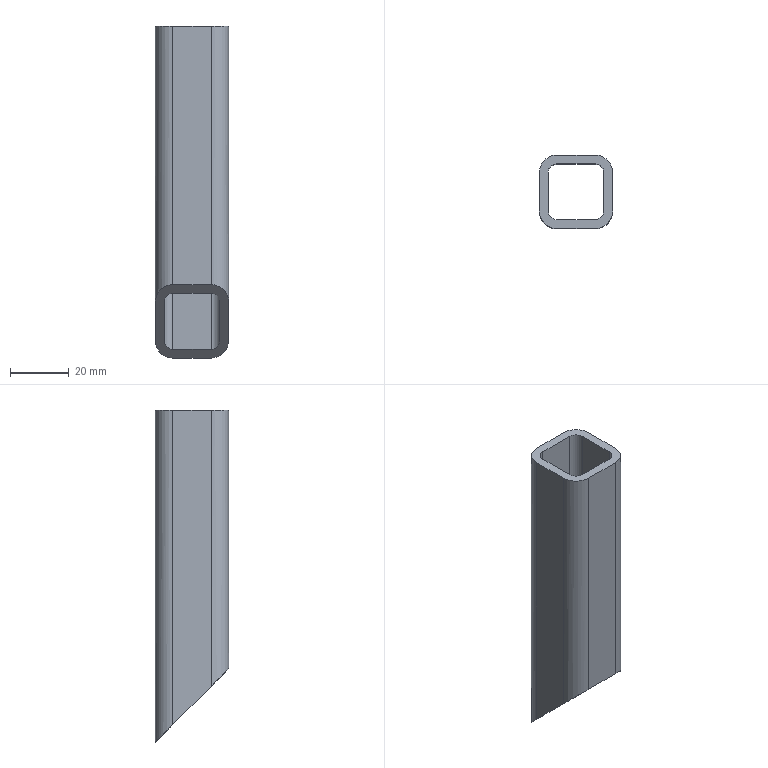Part | STEP file | ISO 10799-2 25x25x3 1784907954311 | 1 solid | 18 faces | box 25 x 25 x 113.072 mm | volume 24220 mm3 | plane 10 | cylinder 8 | commonest cylinder face diameters 6 x4 12 x4
STEP:
#1=CARTESIAN_POINT('',(12.5,-6.5,6.5));
#2=VERTEX_POINT('',#1);
#3=CARTESIAN_POINT('',(12.5,6.5,-6.5));
#4=VERTEX_POINT('',#3);
#5=CARTESIAN_POINT('',(12.5,1.625,-1.625));
#6=DIRECTION('',(0.,0.7071,-0.7071));
#7=VECTOR('',#6,10.);
#8=LINE('',#5,#7);
#9=EDGE_CURVE('',#2,#4,#8,.T.);
#10=ORIENTED_EDGE('',*,*,#9,.F.);
#11=CARTESIAN_POINT('',(6.5,-12.5,12.5));
#12=VERTEX_POINT('',#11);
#13=CARTESIAN_POINT('',(6.5,-6.5,6.5));
#14=DIRECTION('',(0.,0.7071,0.7071));
#15=DIRECTION('',(0.,0.7071,-0.7071));
#16=AXIS2_PLACEMENT_3D('',#13,#14,#15);
#17=ELLIPSE('',#16,8.485,6.);
#18=EDGE_CURVE('',#12,#2,#17,.T.);
#19=ORIENTED_EDGE('',*,*,#18,.F.);
#20=CARTESIAN_POINT('',(-6.5,-12.5,12.5));
#21=VERTEX_POINT('',#20);
#22=CARTESIAN_POINT('',(3.25,-12.5,12.5));
#23=DIRECTION('',(1.,0.,0.));
#24=VECTOR('',#23,10.);
#25=LINE('',#22,#24);
#26=EDGE_CURVE('',#21,#12,#25,.T.);
#27=ORIENTED_EDGE('',*,*,#26,.F.);
#28=CARTESIAN_POINT('',(-12.5,-6.5,6.5));
#29=VERTEX_POINT('',#28);
#30=CARTESIAN_POINT('',(-6.5,-6.5,6.5));
#31=DIRECTION('',(0.,0.7071,0.7071));
#32=DIRECTION('',(0.,0.7071,-0.7071));
#33=AXIS2_PLACEMENT_3D('',#30,#31,#32);
#34=ELLIPSE('',#33,8.485,6.);
#35=EDGE_CURVE('',#29,#21,#34,.T.);
#36=ORIENTED_EDGE('',*,*,#35,.F.);
#37=CARTESIAN_POINT('',(-12.5,6.5,-6.5));
#38=VERTEX_POINT('',#37);
#39=CARTESIAN_POINT('',(-12.5,-1.625,1.625));
#40=DIRECTION('',(0.,-0.7071,0.7071));
#41=VECTOR('',#40,10.);
#42=LINE('',#39,#41);
#43=EDGE_CURVE('',#38,#29,#42,.T.);
#44=ORIENTED_EDGE('',*,*,#43,.F.);
#45=CARTESIAN_POINT('',(-6.5,12.5,-12.5));
#46=VERTEX_POINT('',#45);
#47=CARTESIAN_POINT('',(-6.5,6.5,-6.5));
#48=DIRECTION('',(0.,0.7071,0.7071));
#49=DIRECTION('',(0.,-0.7071,0.7071));
#50=AXIS2_PLACEMENT_3D('',#47,#48,#49);
#51=ELLIPSE('',#50,8.485,6.);
#52=EDGE_CURVE('',#46,#38,#51,.T.);
#53=ORIENTED_EDGE('',*,*,#52,.F.);
#54=CARTESIAN_POINT('',(6.5,12.5,-12.5));
#55=VERTEX_POINT('',#54);
#56=CARTESIAN_POINT('',(-3.25,12.5,-12.5));
#57=DIRECTION('',(1.,0.,0.));
#58=VECTOR('',#57,10.);
#59=LINE('',#56,#58);
#60=EDGE_CURVE('',#46,#55,#59,.T.);
#61=ORIENTED_EDGE('',*,*,#60,.T.);
#62=CARTESIAN_POINT('',(6.5,6.5,-6.5));
#63=DIRECTION('',(0.,0.7071,0.7071));
#64=DIRECTION('',(0.,-0.7071,0.7071));
#65=AXIS2_PLACEMENT_3D('',#62,#63,#64);
#66=ELLIPSE('',#65,8.485,6.);
#67=EDGE_CURVE('',#4,#55,#66,.T.);
#68=ORIENTED_EDGE('',*,*,#67,.F.);
#69=EDGE_LOOP('',(#10,#19,#27,#36,#44,#53,#61,#68));
#70=FACE_OUTER_BOUND('',#69,.T.);
#71=CARTESIAN_POINT('',(6.5,-9.5,9.5));
#72=VERTEX_POINT('',#71);
#73=CARTESIAN_POINT('',(-6.5,-9.5,9.5));
#74=VERTEX_POINT('',#73);
#75=CARTESIAN_POINT('',(3.25,-9.5,9.5));
#76=DIRECTION('',(-1.,0.,0.));
#77=VECTOR('',#76,10.);
#78=LINE('',#75,#77);
#79=EDGE_CURVE('',#72,#74,#78,.T.);
#80=ORIENTED_EDGE('',*,*,#79,.F.);
#81=CARTESIAN_POINT('',(9.5,-6.5,6.5));
#82=VERTEX_POINT('',#81);
#83=CARTESIAN_POINT('',(6.5,-6.5,6.5));
#84=DIRECTION('',(0.,-0.7071,-0.7071));
#85=DIRECTION('',(0.,0.7071,-0.7071));
#86=AXIS2_PLACEMENT_3D('',#83,#84,#85);
#87=ELLIPSE('',#86,4.243,3.);
#88=EDGE_CURVE('',#82,#72,#87,.T.);
#89=ORIENTED_EDGE('',*,*,#88,.F.);
#90=CARTESIAN_POINT('',(9.5,6.5,-6.5));
#91=VERTEX_POINT('',#90);
#92=CARTESIAN_POINT('',(9.5,1.625,-1.625));
#93=DIRECTION('',(0.,-0.7071,0.7071));
#94=VECTOR('',#93,10.);
#95=LINE('',#92,#94);
#96=EDGE_CURVE('',#91,#82,#95,.T.);
#97=ORIENTED_EDGE('',*,*,#96,.F.);
#98=CARTESIAN_POINT('',(6.5,9.5,-9.5));
#99=VERTEX_POINT('',#98);
#100=CARTESIAN_POINT('',(6.5,6.5,-6.5));
#101=DIRECTION('',(0.,-0.7071,-0.7071));
#102=DIRECTION('',(0.,-0.7071,0.7071));
#103=AXIS2_PLACEMENT_3D('',#100,#101,#102);
#104=ELLIPSE('',#103,4.243,3.);
#105=EDGE_CURVE('',#99,#91,#104,.T.);
#106=ORIENTED_EDGE('',*,*,#105,.F.);
#107=CARTESIAN_POINT('',(-6.5,9.5,-9.5));
#108=VERTEX_POINT('',#107);
#109=CARTESIAN_POINT('',(-3.25,9.5,-9.5));
#110=DIRECTION('',(1.,0.,0.));
#111=VECTOR('',#110,10.);
#112=LINE('',#109,#111);
#113=EDGE_CURVE('',#108,#99,#112,.T.);
#114=ORIENTED_EDGE('',*,*,#113,.F.);
#115=CARTESIAN_POINT('',(-9.5,6.5,-6.5));
#116=VERTEX_POINT('',#115);
#117=CARTESIAN_POINT('',(-6.5,6.5,-6.5));
#118=DIRECTION('',(0.,-0.7071,-0.7071));
#119=DIRECTION('',(0.,-0.7071,0.7071));
#120=AXIS2_PLACEMENT_3D('',#117,#118,#119);
#121=ELLIPSE('',#120,4.243,3.);
#122=EDGE_CURVE('',#116,#108,#121,.T.);
#123=ORIENTED_EDGE('',*,*,#122,.F.);
#124=CARTESIAN_POINT('',(-9.5,-6.5,6.5));
#125=VERTEX_POINT('',#124);
#126=CARTESIAN_POINT('',(-9.5,-1.625,1.625));
#127=DIRECTION('',(0.,0.7071,-0.7071));
#128=VECTOR('',#127,10.);
#129=LINE('',#126,#128);
#130=EDGE_CURVE('',#125,#116,#129,.T.);
#131=ORIENTED_EDGE('',*,*,#130,.F.);
#132=CARTESIAN_POINT('',(-6.5,-6.5,6.5));
#133=DIRECTION('',(0.,-0.7071,-0.7071));
#134=DIRECTION('',(0.,0.7071,-0.7071));
#135=AXIS2_PLACEMENT_3D('',#132,#133,#134);
#136=ELLIPSE('',#135,4.243,3.);
#137=EDGE_CURVE('',#74,#125,#136,.T.);
#138=ORIENTED_EDGE('',*,*,#137,.F.);
#139=EDGE_LOOP('',(#80,#89,#97,#106,#114,#123,#131,#138));
#140=FACE_BOUND('',#139,.T.);
#141=CARTESIAN_POINT('',(0.,0.,0.));
#142=DIRECTION('',(0.,0.7071,0.7071));
#143=DIRECTION('',(1.,0.,0.));
#144=AXIS2_PLACEMENT_3D('',#141,#142,#143);
#145=PLANE('',#144);
#146=ADVANCED_FACE('',(#70,#140),#145,.F.);
#147=ORIENTED_EDGE('',*,*,#113,.T.);
#148=CARTESIAN_POINT('',(6.5,9.5,100.572));
#149=VERTEX_POINT('',#148);
#150=CARTESIAN_POINT('',(6.5,9.5,0.));
#151=DIRECTION('',(0.,0.,-1.));
#152=VECTOR('',#151,10.);
#153=LINE('',#150,#152);
#154=EDGE_CURVE('',#149,#99,#153,.T.);
#155=ORIENTED_EDGE('',*,*,#154,.F.);
#156=CARTESIAN_POINT('',(-6.5,9.5,100.572));
#157=VERTEX_POINT('',#156);
#158=CARTESIAN_POINT('',(-3.25,9.5,100.572));
#159=DIRECTION('',(-1.,0.,0.));
#160=VECTOR('',#159,10.);
#161=LINE('',#158,#160);
#162=EDGE_CURVE('',#149,#157,#161,.T.);
#163=ORIENTED_EDGE('',*,*,#162,.T.);
#164=CARTESIAN_POINT('',(-6.5,9.5,0.));
#165=DIRECTION('',(0.,0.,-1.));
#166=VECTOR('',#165,10.);
#167=LINE('',#164,#166);
#168=EDGE_CURVE('',#157,#108,#167,.T.);
#169=ORIENTED_EDGE('',*,*,#168,.T.);
#170=EDGE_LOOP('',(#147,#155,#163,#169));
#171=FACE_OUTER_BOUND('',#170,.T.);
#172=CARTESIAN_POINT('',(-6.5,9.5,0.));
#173=DIRECTION('',(0.,1.,0.));
#174=DIRECTION('',(0.,0.,1.));
#175=AXIS2_PLACEMENT_3D('',#172,#173,#174);
#176=PLANE('',#175);
#177=ADVANCED_FACE('',(#171),#176,.F.);
#178=ORIENTED_EDGE('',*,*,#105,.T.);
#179=CARTESIAN_POINT('',(9.5,6.5,100.572));
#180=VERTEX_POINT('',#179);
#181=CARTESIAN_POINT('',(9.5,6.5,0.));
#182=DIRECTION('',(0.,0.,-1.));
#183=VECTOR('',#182,10.);
#184=LINE('',#181,#183);
#185=EDGE_CURVE('',#180,#91,#184,.T.);
#186=ORIENTED_EDGE('',*,*,#185,.F.);
#187=CARTESIAN_POINT('',(6.5,6.5,100.572));
#188=DIRECTION('',(0.,0.,1.));
#189=DIRECTION('',(-1.,0.,0.));
#190=AXIS2_PLACEMENT_3D('',#187,#188,#189);
#191=CIRCLE('',#190,3.);
#192=EDGE_CURVE('',#180,#149,#191,.T.);
#193=ORIENTED_EDGE('',*,*,#192,.T.);
#194=ORIENTED_EDGE('',*,*,#154,.T.);
#195=EDGE_LOOP('',(#178,#186,#193,#194));
#196=FACE_OUTER_BOUND('',#195,.T.);
#197=CARTESIAN_POINT('',(6.5,6.5,0.));
#198=DIRECTION('',(0.,0.,1.));
#199=DIRECTION('',(-1.,0.,0.));
#200=AXIS2_PLACEMENT_3D('',#197,#198,#199);
#201=CYLINDRICAL_SURFACE('',#200,3.);
#202=ADVANCED_FACE('',(#196),#201,.F.);
#203=ORIENTED_EDGE('',*,*,#96,.T.);
#204=CARTESIAN_POINT('',(9.5,-6.5,100.572));
#205=VERTEX_POINT('',#204);
#206=CARTESIAN_POINT('',(9.5,-6.5,0.));
#207=DIRECTION('',(0.,0.,-1.));
#208=VECTOR('',#207,10.);
#209=LINE('',#206,#208);
#210=EDGE_CURVE('',#205,#82,#209,.T.);
#211=ORIENTED_EDGE('',*,*,#210,.F.);
#212=CARTESIAN_POINT('',(9.5,3.25,100.572));
#213=DIRECTION('',(0.,1.,0.));
#214=VECTOR('',#213,10.);
#215=LINE('',#212,#214);
#216=EDGE_CURVE('',#205,#180,#215,.T.);
#217=ORIENTED_EDGE('',*,*,#216,.T.);
#218=ORIENTED_EDGE('',*,*,#185,.T.);
#219=EDGE_LOOP('',(#203,#211,#217,#218));
#220=FACE_OUTER_BOUND('',#219,.T.);
#221=CARTESIAN_POINT('',(9.5,6.5,0.));
#222=DIRECTION('',(1.,0.,0.));
#223=DIRECTION('',(0.,0.,-1.));
#224=AXIS2_PLACEMENT_3D('',#221,#222,#223);
#225=PLANE('',#224);
#226=ADVANCED_FACE('',(#220),#225,.F.);
#227=ORIENTED_EDGE('',*,*,#88,.T.);
#228=CARTESIAN_POINT('',(6.5,-9.5,100.572));
#229=VERTEX_POINT('',#228);
#230=CARTESIAN_POINT('',(6.5,-9.5,0.));
#231=DIRECTION('',(0.,0.,-1.));
#232=VECTOR('',#231,10.);
#233=LINE('',#230,#232);
#234=EDGE_CURVE('',#229,#72,#233,.T.);
#235=ORIENTED_EDGE('',*,*,#234,.F.);
#236=CARTESIAN_POINT('',(6.5,-6.5,100.572));
#237=DIRECTION('',(0.,0.,1.));
#238=DIRECTION('',(0.,1.,0.));
#239=AXIS2_PLACEMENT_3D('',#236,#237,#238);
#240=CIRCLE('',#239,3.);
#241=EDGE_CURVE('',#229,#205,#240,.T.);
#242=ORIENTED_EDGE('',*,*,#241,.T.);
#243=ORIENTED_EDGE('',*,*,#210,.T.);
#244=EDGE_LOOP('',(#227,#235,#242,#243));
#245=FACE_OUTER_BOUND('',#244,.T.);
#246=CARTESIAN_POINT('',(6.5,-6.5,0.));
#247=DIRECTION('',(0.,0.,1.));
#248=DIRECTION('',(0.,1.,0.));
#249=AXIS2_PLACEMENT_3D('',#246,#247,#248);
#250=CYLINDRICAL_SURFACE('',#249,3.);
#251=ADVANCED_FACE('',(#245),#250,.F.);
#252=ORIENTED_EDGE('',*,*,#43,.T.);
#253=CARTESIAN_POINT('',(-12.5,-6.5,100.572));
#254=VERTEX_POINT('',#253);
#255=CARTESIAN_POINT('',(-12.5,-6.5,0.));
#256=DIRECTION('',(0.,0.,-1.));
#257=VECTOR('',#256,10.);
#258=LINE('',#255,#257);
#259=EDGE_CURVE('',#254,#29,#258,.T.);
#260=ORIENTED_EDGE('',*,*,#259,.F.);
#261=CARTESIAN_POINT('',(-12.5,6.5,100.572));
#262=VERTEX_POINT('',#261);
#263=CARTESIAN_POINT('',(-12.5,-3.25,100.572));
#264=DIRECTION('',(0.,1.,0.));
#265=VECTOR('',#264,10.);
#266=LINE('',#263,#265);
#267=EDGE_CURVE('',#254,#262,#266,.T.);
#268=ORIENTED_EDGE('',*,*,#267,.T.);
#269=CARTESIAN_POINT('',(-12.5,6.5,0.));
#270=DIRECTION('',(0.,0.,-1.));
#271=VECTOR('',#270,10.);
#272=LINE('',#269,#271);
#273=EDGE_CURVE('',#262,#38,#272,.T.);
#274=ORIENTED_EDGE('',*,*,#273,.T.);
#275=EDGE_LOOP('',(#252,#260,#268,#274));
#276=FACE_OUTER_BOUND('',#275,.T.);
#277=CARTESIAN_POINT('',(-12.5,-6.5,0.));
#278=DIRECTION('',(-1.,0.,0.));
#279=DIRECTION('',(0.,0.,1.));
#280=AXIS2_PLACEMENT_3D('',#277,#278,#279);
#281=PLANE('',#280);
#282=ADVANCED_FACE('',(#276),#281,.T.);
#283=ORIENTED_EDGE('',*,*,#35,.T.);
#284=CARTESIAN_POINT('',(-6.5,-12.5,100.572));
#285=VERTEX_POINT('',#284);
#286=CARTESIAN_POINT('',(-6.5,-12.5,0.));
#287=DIRECTION('',(0.,0.,1.));
#288=VECTOR('',#287,10.);
#289=LINE('',#286,#288);
#290=EDGE_CURVE('',#21,#285,#289,.T.);
#291=ORIENTED_EDGE('',*,*,#290,.T.);
#292=CARTESIAN_POINT('',(-6.5,-6.5,100.572));
#293=DIRECTION('',(0.,0.,-1.));
#294=DIRECTION('',(1.,0.,0.));
#295=AXIS2_PLACEMENT_3D('',#292,#293,#294);
#296=CIRCLE('',#295,6.);
#297=EDGE_CURVE('',#285,#254,#296,.T.);
#298=ORIENTED_EDGE('',*,*,#297,.T.);
#299=ORIENTED_EDGE('',*,*,#259,.T.);
#300=EDGE_LOOP('',(#283,#291,#298,#299));
#301=FACE_OUTER_BOUND('',#300,.T.);
#302=CARTESIAN_POINT('',(-6.5,-6.5,0.));
#303=DIRECTION('',(0.,0.,1.));
#304=DIRECTION('',(1.,0.,0.));
#305=AXIS2_PLACEMENT_3D('',#302,#303,#304);
#306=CYLINDRICAL_SURFACE('',#305,6.);
#307=ADVANCED_FACE('',(#301),#306,.T.);
#308=ORIENTED_EDGE('',*,*,#26,.T.);
#309=CARTESIAN_POINT('',(6.5,-12.5,100.572));
#310=VERTEX_POINT('',#309);
#311=CARTESIAN_POINT('',(6.5,-12.5,0.));
#312=DIRECTION('',(0.,0.,-1.));
#313=VECTOR('',#312,10.);
#314=LINE('',#311,#313);
#315=EDGE_CURVE('',#310,#12,#314,.T.);
#316=ORIENTED_EDGE('',*,*,#315,.F.);
#317=CARTESIAN_POINT('',(3.25,-12.5,100.572));
#318=DIRECTION('',(-1.,0.,0.));
#319=VECTOR('',#318,10.);
#320=LINE('',#317,#319);
#321=EDGE_CURVE('',#310,#285,#320,.T.);
#322=ORIENTED_EDGE('',*,*,#321,.T.);
#323=ORIENTED_EDGE('',*,*,#290,.F.);
#324=EDGE_LOOP('',(#308,#316,#322,#323));
#325=FACE_OUTER_BOUND('',#324,.T.);
#326=CARTESIAN_POINT('',(6.5,-12.5,0.));
#327=DIRECTION('',(0.,-1.,0.));
#328=DIRECTION('',(0.,0.,-1.));
#329=AXIS2_PLACEMENT_3D('',#326,#327,#328);
#330=PLANE('',#329);
#331=ADVANCED_FACE('',(#325),#330,.T.);
#332=ORIENTED_EDGE('',*,*,#18,.T.);
#333=CARTESIAN_POINT('',(12.5,-6.5,100.572));
#334=VERTEX_POINT('',#333);
#335=CARTESIAN_POINT('',(12.5,-6.5,0.));
#336=DIRECTION('',(0.,0.,-1.));
#337=VECTOR('',#336,10.);
#338=LINE('',#335,#337);
#339=EDGE_CURVE('',#334,#2,#338,.T.);
#340=ORIENTED_EDGE('',*,*,#339,.F.);
#341=CARTESIAN_POINT('',(6.5,-6.5,100.572));
#342=DIRECTION('',(0.,0.,-1.));
#343=DIRECTION('',(0.,1.,0.));
#344=AXIS2_PLACEMENT_3D('',#341,#342,#343);
#345=CIRCLE('',#344,6.);
#346=EDGE_CURVE('',#334,#310,#345,.T.);
#347=ORIENTED_EDGE('',*,*,#346,.T.);
#348=ORIENTED_EDGE('',*,*,#315,.T.);
#349=EDGE_LOOP('',(#332,#340,#347,#348));
#350=FACE_OUTER_BOUND('',#349,.T.);
#351=CARTESIAN_POINT('',(6.5,-6.5,0.));
#352=DIRECTION('',(0.,0.,1.));
#353=DIRECTION('',(0.,1.,0.));
#354=AXIS2_PLACEMENT_3D('',#351,#352,#353);
#355=CYLINDRICAL_SURFACE('',#354,6.);
#356=ADVANCED_FACE('',(#350),#355,.T.);
#357=ORIENTED_EDGE('',*,*,#79,.T.);
#358=CARTESIAN_POINT('',(-6.5,-9.5,100.572));
#359=VERTEX_POINT('',#358);
#360=CARTESIAN_POINT('',(-6.5,-9.5,0.));
#361=DIRECTION('',(0.,0.,-1.));
#362=VECTOR('',#361,10.);
#363=LINE('',#360,#362);
#364=EDGE_CURVE('',#359,#74,#363,.T.);
#365=ORIENTED_EDGE('',*,*,#364,.F.);
#366=CARTESIAN_POINT('',(3.25,-9.5,100.572));
#367=DIRECTION('',(1.,0.,0.));
#368=VECTOR('',#367,10.);
#369=LINE('',#366,#368);
#370=EDGE_CURVE('',#359,#229,#369,.T.);
#371=ORIENTED_EDGE('',*,*,#370,.T.);
#372=ORIENTED_EDGE('',*,*,#234,.T.);
#373=EDGE_LOOP('',(#357,#365,#371,#372));
#374=FACE_OUTER_BOUND('',#373,.T.);
#375=CARTESIAN_POINT('',(6.5,-9.5,0.));
#376=DIRECTION('',(0.,-1.,0.));
#377=DIRECTION('',(0.,0.,-1.));
#378=AXIS2_PLACEMENT_3D('',#375,#376,#377);
#379=PLANE('',#378);
#380=ADVANCED_FACE('',(#374),#379,.F.);
#381=ORIENTED_EDGE('',*,*,#9,.T.);
#382=CARTESIAN_POINT('',(12.5,6.5,100.572));
#383=VERTEX_POINT('',#382);
#384=CARTESIAN_POINT('',(12.5,6.5,0.));
#385=DIRECTION('',(0.,0.,-1.));
#386=VECTOR('',#385,10.);
#387=LINE('',#384,#386);
#388=EDGE_CURVE('',#383,#4,#387,.T.);
#389=ORIENTED_EDGE('',*,*,#388,.F.);
#390=CARTESIAN_POINT('',(12.5,3.25,100.572));
#391=DIRECTION('',(0.,-1.,0.));
#392=VECTOR('',#391,10.);
#393=LINE('',#390,#392);
#394=EDGE_CURVE('',#383,#334,#393,.T.);
#395=ORIENTED_EDGE('',*,*,#394,.T.);
#396=ORIENTED_EDGE('',*,*,#339,.T.);
#397=EDGE_LOOP('',(#381,#389,#395,#396));
#398=FACE_OUTER_BOUND('',#397,.T.);
#399=CARTESIAN_POINT('',(12.5,6.5,0.));
#400=DIRECTION('',(1.,0.,0.));
#401=DIRECTION('',(0.,0.,-1.));
#402=AXIS2_PLACEMENT_3D('',#399,#400,#401);
#403=PLANE('',#402);
#404=ADVANCED_FACE('',(#398),#403,.T.);
#405=ORIENTED_EDGE('',*,*,#137,.T.);
#406=CARTESIAN_POINT('',(-9.5,-6.5,100.572));
#407=VERTEX_POINT('',#406);
#408=CARTESIAN_POINT('',(-9.5,-6.5,0.));
#409=DIRECTION('',(0.,0.,-1.));
#410=VECTOR('',#409,10.);
#411=LINE('',#408,#410);
#412=EDGE_CURVE('',#407,#125,#411,.T.);
#413=ORIENTED_EDGE('',*,*,#412,.F.);
#414=CARTESIAN_POINT('',(-6.5,-6.5,100.572));
#415=DIRECTION('',(0.,0.,1.));
#416=DIRECTION('',(1.,0.,0.));
#417=AXIS2_PLACEMENT_3D('',#414,#415,#416);
#418=CIRCLE('',#417,3.);
#419=EDGE_CURVE('',#407,#359,#418,.T.);
#420=ORIENTED_EDGE('',*,*,#419,.T.);
#421=ORIENTED_EDGE('',*,*,#364,.T.);
#422=EDGE_LOOP('',(#405,#413,#420,#421));
#423=FACE_OUTER_BOUND('',#422,.T.);
#424=CARTESIAN_POINT('',(-6.5,-6.5,0.));
#425=DIRECTION('',(0.,0.,1.));
#426=DIRECTION('',(1.,0.,0.));
#427=AXIS2_PLACEMENT_3D('',#424,#425,#426);
#428=CYLINDRICAL_SURFACE('',#427,3.);
#429=ADVANCED_FACE('',(#423),#428,.F.);
#430=ORIENTED_EDGE('',*,*,#130,.T.);
#431=CARTESIAN_POINT('',(-9.5,6.5,100.572));
#432=VERTEX_POINT('',#431);
#433=CARTESIAN_POINT('',(-9.5,6.5,0.));
#434=DIRECTION('',(0.,0.,1.));
#435=VECTOR('',#434,10.);
#436=LINE('',#433,#435);
#437=EDGE_CURVE('',#116,#432,#436,.T.);
#438=ORIENTED_EDGE('',*,*,#437,.T.);
#439=CARTESIAN_POINT('',(-9.5,-3.25,100.572));
#440=DIRECTION('',(0.,-1.,0.));
#441=VECTOR('',#440,10.);
#442=LINE('',#439,#441);
#443=EDGE_CURVE('',#432,#407,#442,.T.);
#444=ORIENTED_EDGE('',*,*,#443,.T.);
#445=ORIENTED_EDGE('',*,*,#412,.T.);
#446=EDGE_LOOP('',(#430,#438,#444,#445));
#447=FACE_OUTER_BOUND('',#446,.T.);
#448=CARTESIAN_POINT('',(-9.5,-6.5,0.));
#449=DIRECTION('',(-1.,0.,0.));
#450=DIRECTION('',(0.,0.,1.));
#451=AXIS2_PLACEMENT_3D('',#448,#449,#450);
#452=PLANE('',#451);
#453=ADVANCED_FACE('',(#447),#452,.F.);
#454=ORIENTED_EDGE('',*,*,#122,.T.);
#455=ORIENTED_EDGE('',*,*,#168,.F.);
#456=CARTESIAN_POINT('',(-6.5,6.5,100.572));
#457=DIRECTION('',(0.,0.,1.));
#458=DIRECTION('',(0.,-1.,0.));
#459=AXIS2_PLACEMENT_3D('',#456,#457,#458);
#460=CIRCLE('',#459,3.);
#461=EDGE_CURVE('',#157,#432,#460,.T.);
#462=ORIENTED_EDGE('',*,*,#461,.T.);
#463=ORIENTED_EDGE('',*,*,#437,.F.);
#464=EDGE_LOOP('',(#454,#455,#462,#463));
#465=FACE_OUTER_BOUND('',#464,.T.);
#466=CARTESIAN_POINT('',(-6.5,6.5,0.));
#467=DIRECTION('',(0.,0.,1.));
#468=DIRECTION('',(0.,-1.,0.));
#469=AXIS2_PLACEMENT_3D('',#466,#467,#468);
#470=CYLINDRICAL_SURFACE('',#469,3.);
#471=ADVANCED_FACE('',(#465),#470,.F.);
#472=ORIENTED_EDGE('',*,*,#52,.T.);
#473=ORIENTED_EDGE('',*,*,#273,.F.);
#474=CARTESIAN_POINT('',(-6.5,12.5,100.572));
#475=VERTEX_POINT('',#474);
#476=CARTESIAN_POINT('',(-6.5,6.5,100.572));
#477=DIRECTION('',(0.,0.,-1.));
#478=DIRECTION('',(0.,-1.,0.));
#479=AXIS2_PLACEMENT_3D('',#476,#477,#478);
#480=CIRCLE('',#479,6.);
#481=EDGE_CURVE('',#262,#475,#480,.T.);
#482=ORIENTED_EDGE('',*,*,#481,.T.);
#483=CARTESIAN_POINT('',(-6.5,12.5,0.));
#484=DIRECTION('',(0.,0.,-1.));
#485=VECTOR('',#484,10.);
#486=LINE('',#483,#485);
#487=EDGE_CURVE('',#475,#46,#486,.T.);
#488=ORIENTED_EDGE('',*,*,#487,.T.);
#489=EDGE_LOOP('',(#472,#473,#482,#488));
#490=FACE_OUTER_BOUND('',#489,.T.);
#491=CARTESIAN_POINT('',(-6.5,6.5,0.));
#492=DIRECTION('',(0.,0.,1.));
#493=DIRECTION('',(0.,-1.,0.));
#494=AXIS2_PLACEMENT_3D('',#491,#492,#493);
#495=CYLINDRICAL_SURFACE('',#494,6.);
#496=ADVANCED_FACE('',(#490),#495,.T.);
#497=CARTESIAN_POINT('',(6.5,12.5,100.572));
#498=VERTEX_POINT('',#497);
#499=CARTESIAN_POINT('',(-3.25,12.5,100.572));
#500=DIRECTION('',(1.,0.,0.));
#501=VECTOR('',#500,10.);
#502=LINE('',#499,#501);
#503=EDGE_CURVE('',#475,#498,#502,.T.);
#504=ORIENTED_EDGE('',*,*,#503,.T.);
#505=CARTESIAN_POINT('',(6.5,12.5,0.));
#506=DIRECTION('',(0.,0.,-1.));
#507=VECTOR('',#506,10.);
#508=LINE('',#505,#507);
#509=EDGE_CURVE('',#498,#55,#508,.T.);
#510=ORIENTED_EDGE('',*,*,#509,.T.);
#511=ORIENTED_EDGE('',*,*,#60,.F.);
#512=ORIENTED_EDGE('',*,*,#487,.F.);
#513=EDGE_LOOP('',(#504,#510,#511,#512));
#514=FACE_OUTER_BOUND('',#513,.T.);
#515=CARTESIAN_POINT('',(-6.5,12.5,0.));
#516=DIRECTION('',(0.,1.,0.));
#517=DIRECTION('',(0.,0.,1.));
#518=AXIS2_PLACEMENT_3D('',#515,#516,#517);
#519=PLANE('',#518);
#520=ADVANCED_FACE('',(#514),#519,.T.);
#521=ORIENTED_EDGE('',*,*,#67,.T.);
#522=ORIENTED_EDGE('',*,*,#509,.F.);
#523=CARTESIAN_POINT('',(6.5,6.5,100.572));
#524=DIRECTION('',(0.,0.,-1.));
#525=DIRECTION('',(-1.,0.,0.));
#526=AXIS2_PLACEMENT_3D('',#523,#524,#525);
#527=CIRCLE('',#526,6.);
#528=EDGE_CURVE('',#498,#383,#527,.T.);
#529=ORIENTED_EDGE('',*,*,#528,.T.);
#530=ORIENTED_EDGE('',*,*,#388,.T.);
#531=EDGE_LOOP('',(#521,#522,#529,#530));
#532=FACE_OUTER_BOUND('',#531,.T.);
#533=CARTESIAN_POINT('',(6.5,6.5,0.));
#534=DIRECTION('',(0.,0.,1.));
#535=DIRECTION('',(-1.,0.,0.));
#536=AXIS2_PLACEMENT_3D('',#533,#534,#535);
#537=CYLINDRICAL_SURFACE('',#536,6.);
#538=ADVANCED_FACE('',(#532),#537,.T.);
#539=ORIENTED_EDGE('',*,*,#267,.F.);
#540=ORIENTED_EDGE('',*,*,#297,.F.);
#541=ORIENTED_EDGE('',*,*,#321,.F.);
#542=ORIENTED_EDGE('',*,*,#346,.F.);
#543=ORIENTED_EDGE('',*,*,#394,.F.);
#544=ORIENTED_EDGE('',*,*,#528,.F.);
#545=ORIENTED_EDGE('',*,*,#503,.F.);
#546=ORIENTED_EDGE('',*,*,#481,.F.);
#547=EDGE_LOOP('',(#539,#540,#541,#542,#543,#544,#545,#546));
#548=FACE_OUTER_BOUND('',#547,.T.);
#549=ORIENTED_EDGE('',*,*,#162,.F.);
#550=ORIENTED_EDGE('',*,*,#192,.F.);
#551=ORIENTED_EDGE('',*,*,#216,.F.);
#552=ORIENTED_EDGE('',*,*,#241,.F.);
#553=ORIENTED_EDGE('',*,*,#370,.F.);
#554=ORIENTED_EDGE('',*,*,#419,.F.);
#555=ORIENTED_EDGE('',*,*,#443,.F.);
#556=ORIENTED_EDGE('',*,*,#461,.F.);
#557=EDGE_LOOP('',(#549,#550,#551,#552,#553,#554,#555,#556));
#558=FACE_BOUND('',#557,.T.);
#559=CARTESIAN_POINT('',(0.,0.,100.572));
#560=DIRECTION('',(0.,0.,1.));
#561=DIRECTION('',(1.,0.,0.));
#562=AXIS2_PLACEMENT_3D('',#559,#560,#561);
#563=PLANE('',#562);
#564=ADVANCED_FACE('',(#548,#558),#563,.T.);
#565=CLOSED_SHELL('',(#146,#177,#202,#226,#251,#282,#307,#331,#356,#380,#404,#429,#453,#471,#496,#520,#538,#564));
#566=MANIFOLD_SOLID_BREP('',#565);
#567=(LENGTH_UNIT()NAMED_UNIT(*)SI_UNIT(.MILLI.,.METRE.));
#568=UNCERTAINTY_MEASURE_WITH_UNIT(LENGTH_MEASURE(0.01),#567,'','');
#569=(NAMED_UNIT(*)PLANE_ANGLE_UNIT()SI_UNIT($,.RADIAN.));
#570=(NAMED_UNIT(*)SI_UNIT($,.STERADIAN.)SOLID_ANGLE_UNIT());
#571=(GEOMETRIC_REPRESENTATION_CONTEXT(3)GLOBAL_UNCERTAINTY_ASSIGNED_CONTEXT((#568))GLOBAL_UNIT_ASSIGNED_CONTEXT((#567,#569,#570))REPRESENTATION_CONTEXT('',''));
#572=ADVANCED_BREP_SHAPE_REPRESENTATION('',(#566),#571);